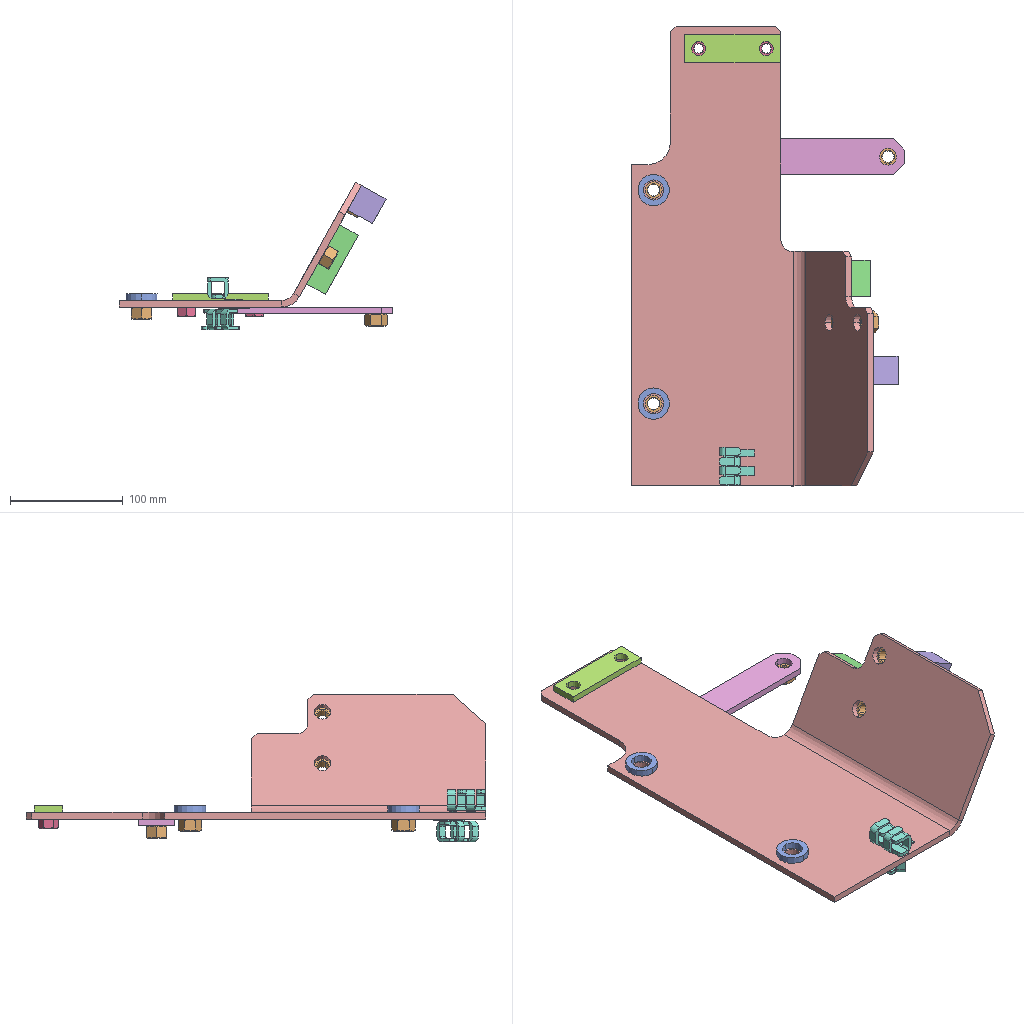Assembly | SolidWorks | 8 different items | 16 placed | box 243 x 408 x 131 mm
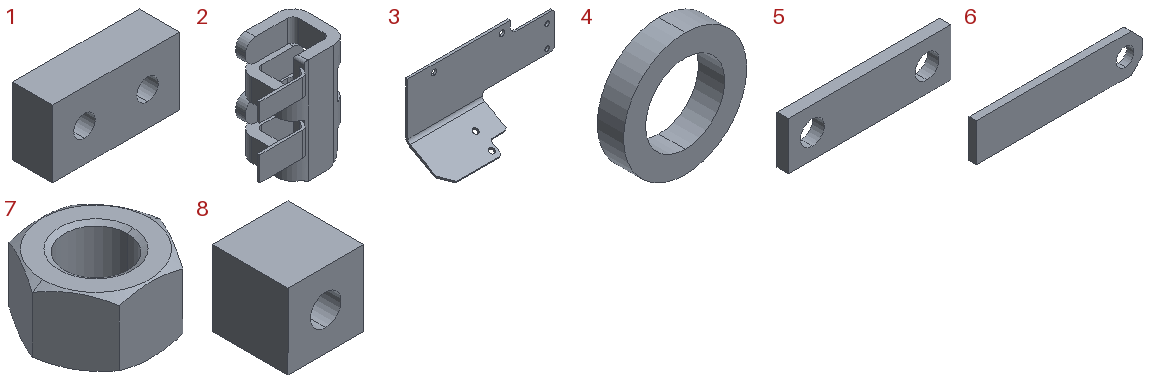Parts list (item | quantity | size | volume | features):
1 | x1 | 60 x 19 x 32 mm | 33375 mm3 | features FlatPattern 1, HoleWzd 1, SMBaseFlange 1, SheetMetal 1
2 | x2 | 31.262 x 20.2 x 34.4 mm | 4311 mm3 | features MBimport 1
3 | x1 | 408 x 110.914 x 215 mm | 454933 mm3 | features ICE 2, Chamfer 1, FlatPattern 1, SMBaseFlange 1, SheetMetal 1
4 | x2 | 28 x 6 x 28 mm | 2168 mm3 | features FlatPattern 1, SMBaseFlange 1, SheetMetal 1
5 | x1 | 85 x 6 x 25 mm | 11277 mm3 | features FlatPattern 1, SMBaseFlange 1, SheetMetal 1
6 | x1 | 140 x 6 x 32 mm | 25220 mm3 | features FlatPattern 1, SMBaseFlange 1, SheetMetal 1
7 | x7 | 27.713 x 24 x 14.8 mm | 5071 mm3 | features RevCut 2, Chamfer 1, Extrusion 1, LPattern 1
8 | x1 | 25 x 25 x 25 mm | 13582 mm3 | features Extrusion 1, HoleWzd 1
Mates (type | each side: item.copy, entity, surface, feature):
Coincident | 3.1 face plane Base-Flange1 | 4.1 face plane Base-Flange1
Concentric | 3.1 face cylinder Cut-Extrude1 | 4.1 face cylinder Base-Flange1
Parallel | 4.1 plane | assembly plane
Coincident | 3.1 face plane Base-Flange1 | 5.1 face plane Base-Flange1
Concentric | 3.1 face cylinder Cut-Extrude1 | 5.1 face cylinder Base-Flange1 | 2 times
Coincident | 3.1 face plane Base-Flange1 | 2.1 face plane 08036-D1630.STEP
DistanceDim | 3.1 face plane Base-Flange1 | 2.1 face plane 08036-D1630.STEP
DistanceDim | 2.1 face plane 08036-D1630.STEP | 3.1 face plane Base-Flange1
Concentric | 3.1 face cylinder Cut-Extrude1 | 7.1 face cone EndChamfer
Coincident | 3.1 face plane Base-Flange1 | 7.1 face plane BaseNut
Concentric | 3.1 face cylinder Cut-Extrude1 | 7.2 face cone EndChamfer
Coincident | 3.1 face plane Base-Flange1 | 7.2 face plane BaseNut
Parallel | 3.1 face plane Base-Flange1 | 7.1 face plane BaseNut
Parallel | 3.1 face plane Base-Flange1 | 7.2 face plane BaseNut
Coincident | 3.1 face plane Base-Flange1 | 1.1 face plane Base-Flange1
Coincident | 3.1 face plane Cut-Extrude2 | 1.1 face plane Base-Flange1
DistanceDim | 1.1 face cylinder M12 Tapped Hole1 | 3.1 face plane Base-Flange1
Concentric | 3.1 face cylinder Cut-Extrude2 | 7.3 face cone EndChamfer
Coincident | 3.1 face plane Base-Flange1 | 7.3 face plane BaseNut
Coincident | 3.1 face plane Base-Flange1 | 7.4 face plane BaseNut
Concentric | 3.1 face cylinder Cut-Extrude2 | 7.4 face cylinder BaseNut
Parallel | 7.4 face plane BaseNut | 3.1 face plane Base-Flange1
Parallel | 3.1 face plane Base-Flange1 | 7.3 face plane BaseNut
Coincident | 3.1 face plane Base-Flange1 | 8.1 face plane Boss-Extrude1 | 2 times
DistanceDim | 3.1 face plane Cut-Extrude2 | 8.1 face cylinder M12 Tapped Hole1
Coincident | 3.1 face plane Base-Flange1 | 6.1 face plane Base-Flange1
DistanceDim | 3.1 face plane Base-Flange1 | 6.1 face cylinder Base-Flange1 | 2 times
Concentric | 3.1 face cylinder Cut-Extrude1 | 7.5 face cone EndChamfer
Coincident | 3.1 face plane Base-Flange1 | 7.5 face plane BaseNut
Concentric | 3.1 face cylinder Cut-Extrude1 | 7.6 face cone EndChamfer
Coincident | 3.1 face plane Base-Flange1 | 7.6 face plane BaseNut
Parallel | 3.1 face plane Cut-Extrude1 | 7.6 face plane BaseNut
Parallel | 3.1 face plane Cut-Extrude1 | 7.5 face plane BaseNut
Parallel | 3.1 face plane Cut-Extrude1 | 6.1 face plane Base-Flange1
Concentric | 6.1 face cylinder Base-Flange1 | 7.7 face cone EndChamfer
Coincident | 6.1 face plane Base-Flange1 | 7.7 face plane BaseNut
Parallel | 7.7 face plane BaseNut | assembly plane
Coincident | 3.1 face plane Base-Flange1 | 2.2 face plane 08036-D1630.STEP
PlanarAngleDim | 2.2 face plane 08036-D1630.STEP | 3.1 face plane Base-Flange1
DistanceDim | 3.1 face plane Base-Flange1 | 2.2 vertex
DistanceDim | 2.2 vertex | 3.1 face plane Base-Flange1